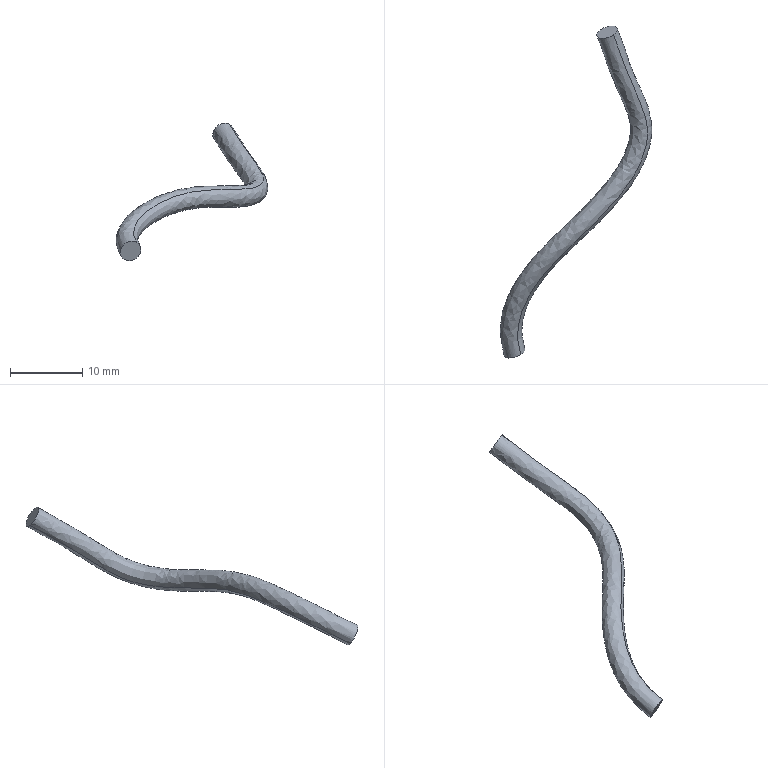Part | SolidWorks | features BaseBody 1 | 1 solid | 4 faces | box 20.926 x 45.783 x 18.973 mm | volume 386.348 mm3 | spline 2 | plane 2
STEP:
#1=CARTESIAN_POINT('',(1917.914,-205.49,926.821));
#2=VERTEX_POINT('',#1);
#3=CARTESIAN_POINT('',(1919.648,-206.093,929.194));
#4=VERTEX_POINT('',#3);
#5=CARTESIAN_POINT('',(1918.781,-205.792,928.008));
#6=DIRECTION('',(-0.2786,0.8622,0.423));
#7=DIRECTION('',(-0.8971,-0.3909,0.206));
#8=AXIS2_PLACEMENT_3D('',#5,#6,#7);
#9=CIRCLE('',#8,1.5);
#10=EDGE_CURVE('',#2,#4,#9,.T.);
#11=ORIENTED_EDGE('',*,*,#10,.T.);
#12=CARTESIAN_POINT('',(1932.433,-161.972,945.472));
#13=VERTEX_POINT('',#12);
#14=CARTESIAN_POINT('',(1919.648,-206.093,929.194));
#15=CARTESIAN_POINT('',(1919.397,-205.314,929.576));
#16=CARTESIAN_POINT('',(1919.227,-204.52,929.968));
#17=CARTESIAN_POINT('',(1919.15,-203.728,930.363));
#18=CARTESIAN_POINT('',(1919.186,-202.087,931.188));
#19=CARTESIAN_POINT('',(1919.601,-200.464,932.011));
#20=CARTESIAN_POINT('',(1919.911,-199.629,932.434));
#21=CARTESIAN_POINT('',(1920.811,-197.733,933.386));
#22=CARTESIAN_POINT('',(1922.058,-195.931,934.252));
#23=CARTESIAN_POINT('',(1922.857,-194.931,934.712));
#24=CARTESIAN_POINT('',(1924.474,-193.116,935.476));
#25=CARTESIAN_POINT('',(1926.3,-191.332,936.005));
#26=CARTESIAN_POINT('',(1927.167,-190.517,936.18));
#27=CARTESIAN_POINT('',(1929.,-188.796,936.417));
#28=CARTESIAN_POINT('',(1930.791,-187.019,936.47));
#29=CARTESIAN_POINT('',(1931.687,-186.078,936.473));
#30=CARTESIAN_POINT('',(1933.237,-184.33,936.474));
#31=CARTESIAN_POINT('',(1934.618,-182.446,936.536));
#32=CARTESIAN_POINT('',(1935.18,-181.584,936.588));
#33=CARTESIAN_POINT('',(1936.101,-179.958,936.744));
#34=CARTESIAN_POINT('',(1936.743,-178.222,937.066));
#35=CARTESIAN_POINT('',(1936.952,-177.433,937.253));
#36=CARTESIAN_POINT('',(1937.175,-176.026,937.663));
#37=CARTESIAN_POINT('',(1937.115,-174.656,938.205));
#38=CARTESIAN_POINT('',(1937.031,-174.042,938.478));
#39=CARTESIAN_POINT('',(1936.759,-172.889,939.053));
#40=CARTESIAN_POINT('',(1936.351,-171.817,939.673));
#41=CARTESIAN_POINT('',(1936.136,-171.318,939.976));
#42=CARTESIAN_POINT('',(1935.572,-170.072,940.747));
#43=CARTESIAN_POINT('',(1935.003,-168.842,941.516));
#44=CARTESIAN_POINT('',(1934.686,-168.106,941.963));
#45=CARTESIAN_POINT('',(1934.027,-166.419,942.951));
#46=CARTESIAN_POINT('',(1933.433,-164.685,943.918));
#47=CARTESIAN_POINT('',(1933.15,-163.847,944.384));
#48=CARTESIAN_POINT('',(1932.801,-162.904,944.925));
#49=CARTESIAN_POINT('',(1932.433,-161.972,945.472));
#50=B_SPLINE_CURVE_WITH_KNOTS('',5,(#14,#15,#16,#17,#18,#19,#20,#21,#22,#23,#24,#25,#26,#27,#28,#29,#30,#31,#32,#33,#34,#35,#36,#37,#38,#39,#40,#41,#42,#43,#44,#45,#46,#47,#48,#49),.UNSPECIFIED.,.F.,.F.,(6,3,3,3,3,3,3,3,3,3,3,6),(0.,0.08786,0.1809,0.3039,0.4114,0.5244,0.617,0.6949,0.759,0.8151,0.8984,1.),.UNSPECIFIED.);
#51=EDGE_CURVE('',#4,#13,#50,.T.);
#52=ORIENTED_EDGE('',*,*,#51,.T.);
#53=CARTESIAN_POINT('',(1930.669,-161.3,943.14));
#54=VERTEX_POINT('',#53);
#55=CARTESIAN_POINT('',(1931.551,-161.636,944.306));
#56=DIRECTION('',(-0.3234,0.8156,0.4797));
#57=DIRECTION('',(-0.8654,-0.4601,0.1988));
#58=AXIS2_PLACEMENT_3D('',#55,#56,#57);
#59=CIRCLE('',#58,1.5);
#60=EDGE_CURVE('',#54,#13,#59,.T.);
#61=ORIENTED_EDGE('',*,*,#60,.F.);
#62=CARTESIAN_POINT('',(1930.669,-161.3,943.14));
#63=CARTESIAN_POINT('',(1931.037,-162.223,942.595));
#64=CARTESIAN_POINT('',(1931.385,-163.158,942.058));
#65=CARTESIAN_POINT('',(1931.668,-163.991,941.594));
#66=CARTESIAN_POINT('',(1932.262,-165.729,940.624));
#67=CARTESIAN_POINT('',(1932.923,-167.438,939.629));
#68=CARTESIAN_POINT('',(1933.241,-168.186,939.178));
#69=CARTESIAN_POINT('',(1933.811,-169.428,938.405));
#70=CARTESIAN_POINT('',(1934.374,-170.663,937.638));
#71=CARTESIAN_POINT('',(1934.588,-171.151,937.339));
#72=CARTESIAN_POINT('',(1934.994,-172.187,936.731));
#73=CARTESIAN_POINT('',(1935.26,-173.283,936.179));
#74=CARTESIAN_POINT('',(1935.338,-173.863,935.921));
#75=CARTESIAN_POINT('',(1935.382,-175.153,935.42));
#76=CARTESIAN_POINT('',(1935.143,-176.466,935.063));
#77=CARTESIAN_POINT('',(1934.928,-177.199,934.906));
#78=CARTESIAN_POINT('',(1934.286,-178.811,934.646));
#79=CARTESIAN_POINT('',(1933.389,-180.326,934.535));
#80=CARTESIAN_POINT('',(1932.845,-181.133,934.502));
#81=CARTESIAN_POINT('',(1931.516,-182.901,934.472));
#82=CARTESIAN_POINT('',(1930.039,-184.548,934.486));
#83=CARTESIAN_POINT('',(1929.19,-185.433,934.487));
#84=CARTESIAN_POINT('',(1927.513,-187.096,934.438));
#85=CARTESIAN_POINT('',(1925.802,-188.705,934.215));
#86=CARTESIAN_POINT('',(1924.987,-189.47,934.052));
#87=CARTESIAN_POINT('',(1923.219,-191.181,933.558));
#88=CARTESIAN_POINT('',(1921.56,-193.001,932.817));
#89=CARTESIAN_POINT('',(1920.716,-194.028,932.36));
#90=CARTESIAN_POINT('',(1919.361,-195.913,931.486));
#91=CARTESIAN_POINT('',(1918.322,-197.986,930.486));
#92=CARTESIAN_POINT('',(1917.949,-198.919,930.034));
#93=CARTESIAN_POINT('',(1917.424,-200.781,929.127));
#94=CARTESIAN_POINT('',(1917.345,-202.722,928.178));
#95=CARTESIAN_POINT('',(1917.427,-203.663,927.718));
#96=CARTESIAN_POINT('',(1917.624,-204.592,927.262));
#97=CARTESIAN_POINT('',(1917.914,-205.49,926.821));
#98=B_SPLINE_CURVE_WITH_KNOTS('',5,(#62,#63,#64,#65,#66,#67,#68,#69,#70,#71,#72,#73,#74,#75,#76,#77,#78,#79,#80,#81,#82,#83,#84,#85,#86,#87,#88,#89,#90,#91,#92,#93,#94,#95,#96,#97),.UNSPECIFIED.,.F.,.F.,(6,3,3,3,3,3,3,3,3,3,3,6),(0.,0.1016,0.1849,0.241,0.3051,0.383,0.4756,0.5886,0.6961,0.8191,0.9121,1.),.UNSPECIFIED.);
#99=EDGE_CURVE('',#54,#2,#98,.T.);
#100=ORIENTED_EDGE('',*,*,#99,.T.);
#101=EDGE_LOOP('',(#11,#52,#61,#100));
#102=FACE_OUTER_BOUND('',#101,.T.);
#103=CARTESIAN_POINT('',(1930.669,-161.3,943.14));
#104=CARTESIAN_POINT('',(1926.22,-164.5,945.581));
#105=CARTESIAN_POINT('',(1931.971,-164.245,949.024));
#106=CARTESIAN_POINT('',(1936.421,-161.045,946.583));
#107=CARTESIAN_POINT('',(1935.119,-158.099,940.699));
#108=CARTESIAN_POINT('',(1930.669,-161.3,943.14));
#109=CARTESIAN_POINT('',(1931.037,-162.223,942.595));
#110=CARTESIAN_POINT('',(1926.553,-165.343,945.079));
#111=CARTESIAN_POINT('',(1932.322,-165.144,948.496));
#112=CARTESIAN_POINT('',(1936.807,-162.024,946.012));
#113=CARTESIAN_POINT('',(1935.521,-159.104,940.112));
#114=CARTESIAN_POINT('',(1931.037,-162.223,942.595));
#115=CARTESIAN_POINT('',(1931.385,-163.158,942.058));
#116=CARTESIAN_POINT('',(1926.864,-166.186,944.59));
#117=CARTESIAN_POINT('',(1932.653,-166.05,947.976));
#118=CARTESIAN_POINT('',(1937.175,-163.022,945.445));
#119=CARTESIAN_POINT('',(1935.906,-160.13,939.526));
#120=CARTESIAN_POINT('',(1931.385,-163.158,942.058));
#121=CARTESIAN_POINT('',(1931.668,-163.991,941.594));
#122=CARTESIAN_POINT('',(1927.127,-166.959,944.156));
#123=CARTESIAN_POINT('',(1932.928,-166.864,947.523));
#124=CARTESIAN_POINT('',(1937.469,-163.895,944.962));
#125=CARTESIAN_POINT('',(1936.209,-161.023,939.032));
#126=CARTESIAN_POINT('',(1931.668,-163.991,941.594));
#127=CARTESIAN_POINT('',(1932.262,-165.729,940.624));
#128=CARTESIAN_POINT('',(1927.74,-168.756,943.157));
#129=CARTESIAN_POINT('',(1933.53,-168.621,946.543));
#130=CARTESIAN_POINT('',(1938.052,-165.595,944.011));
#131=CARTESIAN_POINT('',(1936.785,-162.703,938.092));
#132=CARTESIAN_POINT('',(1932.262,-165.729,940.624));
#133=CARTESIAN_POINT('',(1932.923,-167.438,939.629));
#134=CARTESIAN_POINT('',(1928.496,-170.696,942.04));
#135=CARTESIAN_POINT('',(1934.235,-170.402,945.503));
#136=CARTESIAN_POINT('',(1938.662,-167.144,943.091));
#137=CARTESIAN_POINT('',(1937.351,-164.181,937.218));
#138=CARTESIAN_POINT('',(1932.923,-167.438,939.629));
#139=CARTESIAN_POINT('',(1933.241,-168.186,939.178));
#140=CARTESIAN_POINT('',(1928.867,-171.554,941.529));
#141=CARTESIAN_POINT('',(1934.577,-171.182,945.029));
#142=CARTESIAN_POINT('',(1938.952,-167.814,942.678));
#143=CARTESIAN_POINT('',(1937.615,-164.818,936.827));
#144=CARTESIAN_POINT('',(1933.241,-168.186,939.178));
#145=CARTESIAN_POINT('',(1933.811,-169.428,938.405));
#146=CARTESIAN_POINT('',(1929.495,-172.914,940.691));
#147=CARTESIAN_POINT('',(1935.175,-172.459,944.232));
#148=CARTESIAN_POINT('',(1939.491,-168.973,941.945));
#149=CARTESIAN_POINT('',(1938.127,-165.942,936.118));
#150=CARTESIAN_POINT('',(1933.811,-169.428,938.405));
#151=CARTESIAN_POINT('',(1934.374,-170.663,937.638));
#152=CARTESIAN_POINT('',(1930.003,-174.037,939.986));
#153=CARTESIAN_POINT('',(1935.712,-173.66,943.488));
#154=CARTESIAN_POINT('',(1940.083,-170.286,941.14));
#155=CARTESIAN_POINT('',(1938.745,-167.289,935.29));
#156=CARTESIAN_POINT('',(1934.374,-170.663,937.638));
#157=CARTESIAN_POINT('',(1934.588,-171.151,937.339));
#158=CARTESIAN_POINT('',(1930.168,-174.43,939.739));
#159=CARTESIAN_POINT('',(1935.903,-174.121,943.208));
#160=CARTESIAN_POINT('',(1940.323,-170.843,940.808));
#161=CARTESIAN_POINT('',(1939.008,-167.872,934.938));
#162=CARTESIAN_POINT('',(1934.588,-171.151,937.339));
#163=CARTESIAN_POINT('',(1934.994,-172.187,936.731));
#164=CARTESIAN_POINT('',(1930.408,-175.092,939.331));
#165=CARTESIAN_POINT('',(1936.232,-175.043,942.675));
#166=CARTESIAN_POINT('',(1940.817,-172.138,940.075));
#167=CARTESIAN_POINT('',(1939.579,-169.282,934.131));
#168=CARTESIAN_POINT('',(1934.994,-172.187,936.731));
#169=CARTESIAN_POINT('',(1935.26,-173.283,936.179));
#170=CARTESIAN_POINT('',(1930.491,-175.512,939.107));
#171=CARTESIAN_POINT('',(1936.419,-175.917,942.241));
#172=CARTESIAN_POINT('',(1941.187,-173.688,939.312));
#173=CARTESIAN_POINT('',(1940.028,-171.054,933.25));
#174=CARTESIAN_POINT('',(1935.26,-173.283,936.179));
#175=CARTESIAN_POINT('',(1935.338,-173.863,935.921));
#176=CARTESIAN_POINT('',(1930.505,-175.669,939.041));
#177=CARTESIAN_POINT('',(1936.475,-176.352,942.049));
#178=CARTESIAN_POINT('',(1941.308,-174.546,938.929));
#179=CARTESIAN_POINT('',(1940.17,-172.057,932.801));
#180=CARTESIAN_POINT('',(1935.338,-173.863,935.921));
#181=CARTESIAN_POINT('',(1935.382,-175.153,935.42));
#182=CARTESIAN_POINT('',(1930.528,-175.972,938.951));
#183=CARTESIAN_POINT('',(1936.54,-177.308,941.672));
#184=CARTESIAN_POINT('',(1941.394,-176.489,938.14));
#185=CARTESIAN_POINT('',(1940.236,-174.333,931.888));
#186=CARTESIAN_POINT('',(1935.382,-175.153,935.42));
#187=CARTESIAN_POINT('',(1935.143,-176.466,935.063));
#188=CARTESIAN_POINT('',(1930.508,-176.317,938.934));
#189=CARTESIAN_POINT('',(1936.443,-178.325,941.379));
#190=CARTESIAN_POINT('',(1941.078,-178.475,937.508));
#191=CARTESIAN_POINT('',(1939.778,-176.616,931.191));
#192=CARTESIAN_POINT('',(1935.143,-176.466,935.063));
#193=CARTESIAN_POINT('',(1934.928,-177.199,934.906));
#194=CARTESIAN_POINT('',(1930.478,-176.575,938.923));
#195=CARTESIAN_POINT('',(1936.333,-178.933,941.234));
#196=CARTESIAN_POINT('',(1940.784,-179.557,937.217));
#197=CARTESIAN_POINT('',(1939.379,-177.823,930.889));
#198=CARTESIAN_POINT('',(1934.928,-177.199,934.906));
#199=CARTESIAN_POINT('',(1934.286,-178.811,934.646));
#200=CARTESIAN_POINT('',(1930.27,-177.324,938.903));
#201=CARTESIAN_POINT('',(1935.908,-180.362,940.97));
#202=CARTESIAN_POINT('',(1939.923,-181.849,936.713));
#203=CARTESIAN_POINT('',(1938.302,-180.298,930.388));
#204=CARTESIAN_POINT('',(1934.286,-178.811,934.646));
#205=CARTESIAN_POINT('',(1933.389,-180.326,934.535));
#206=CARTESIAN_POINT('',(1929.775,-178.324,938.902));
#207=CARTESIAN_POINT('',(1935.164,-181.842,940.824));
#208=CARTESIAN_POINT('',(1938.779,-183.844,936.458));
#209=CARTESIAN_POINT('',(1937.004,-182.328,930.168));
#210=CARTESIAN_POINT('',(1933.389,-180.326,934.535));
#211=CARTESIAN_POINT('',(1932.845,-181.133,934.502));
#212=CARTESIAN_POINT('',(1929.415,-178.921,938.909));
#213=CARTESIAN_POINT('',(1934.675,-182.654,940.774));
#214=CARTESIAN_POINT('',(1938.105,-184.866,936.367));
#215=CARTESIAN_POINT('',(1936.275,-183.345,930.095));
#216=CARTESIAN_POINT('',(1932.845,-181.133,934.502));
#217=CARTESIAN_POINT('',(1931.516,-182.901,934.472));
#218=CARTESIAN_POINT('',(1928.43,-180.334,938.943));
#219=CARTESIAN_POINT('',(1933.415,-184.475,940.711));
#220=CARTESIAN_POINT('',(1936.501,-187.042,936.24));
#221=CARTESIAN_POINT('',(1934.602,-185.467,930.002));
#222=CARTESIAN_POINT('',(1931.516,-182.901,934.472));
#223=CARTESIAN_POINT('',(1930.039,-184.548,934.486));
#224=CARTESIAN_POINT('',(1927.129,-181.839,938.98));
#225=CARTESIAN_POINT('',(1931.88,-186.254,940.707));
#226=CARTESIAN_POINT('',(1934.79,-188.963,936.213));
#227=CARTESIAN_POINT('',(1932.949,-187.257,929.991));
#228=CARTESIAN_POINT('',(1930.039,-184.548,934.486));
#229=CARTESIAN_POINT('',(1929.19,-185.433,934.487));
#230=CARTESIAN_POINT('',(1926.328,-182.69,938.99));
#231=CARTESIAN_POINT('',(1930.96,-187.233,940.705));
#232=CARTESIAN_POINT('',(1933.822,-189.977,936.202));
#233=CARTESIAN_POINT('',(1932.052,-188.177,929.984));
#234=CARTESIAN_POINT('',(1929.19,-185.433,934.487));
#235=CARTESIAN_POINT('',(1927.513,-187.096,934.438));
#236=CARTESIAN_POINT('',(1924.631,-184.378,938.947));
#237=CARTESIAN_POINT('',(1929.045,-189.137,940.65));
#238=CARTESIAN_POINT('',(1931.927,-191.854,936.141));
#239=CARTESIAN_POINT('',(1930.395,-189.813,929.928));
#240=CARTESIAN_POINT('',(1927.513,-187.096,934.438));
#241=CARTESIAN_POINT('',(1925.802,-188.705,934.215));
#242=CARTESIAN_POINT('',(1922.685,-186.206,938.695));
#243=CARTESIAN_POINT('',(1926.973,-191.08,940.386));
#244=CARTESIAN_POINT('',(1930.091,-193.579,935.906));
#245=CARTESIAN_POINT('',(1928.92,-191.205,929.734));
#246=CARTESIAN_POINT('',(1925.802,-188.705,934.215));
#247=CARTESIAN_POINT('',(1924.987,-189.47,934.052));
#248=CARTESIAN_POINT('',(1921.706,-187.124,938.505));
#249=CARTESIAN_POINT('',(1925.972,-192.02,940.184));
#250=CARTESIAN_POINT('',(1929.253,-194.366,935.731));
#251=CARTESIAN_POINT('',(1928.268,-191.816,929.599));
#252=CARTESIAN_POINT('',(1924.987,-189.47,934.052));
#253=CARTESIAN_POINT('',(1923.219,-191.181,933.558));
#254=CARTESIAN_POINT('',(1919.572,-189.225,937.925));
#255=CARTESIAN_POINT('',(1923.906,-194.074,939.578));
#256=CARTESIAN_POINT('',(1927.553,-196.03,935.212));
#257=CARTESIAN_POINT('',(1926.866,-193.136,929.191));
#258=CARTESIAN_POINT('',(1923.219,-191.181,933.558));
#259=CARTESIAN_POINT('',(1921.56,-193.001,932.817));
#260=CARTESIAN_POINT('',(1917.581,-191.498,937.065));
#261=CARTESIAN_POINT('',(1922.165,-196.109,938.731));
#262=CARTESIAN_POINT('',(1926.145,-197.612,934.483));
#263=CARTESIAN_POINT('',(1925.539,-194.503,928.568));
#264=CARTESIAN_POINT('',(1921.56,-193.001,932.817));
#265=CARTESIAN_POINT('',(1920.716,-194.028,932.36));
#266=CARTESIAN_POINT('',(1916.579,-192.778,936.541));
#267=CARTESIAN_POINT('',(1921.333,-197.21,938.234));
#268=CARTESIAN_POINT('',(1925.469,-198.46,934.054));
#269=CARTESIAN_POINT('',(1924.852,-195.278,928.18));
#270=CARTESIAN_POINT('',(1920.716,-194.028,932.36));
#271=CARTESIAN_POINT('',(1919.361,-195.913,931.486));
#272=CARTESIAN_POINT('',(1914.956,-195.162,935.526));
#273=CARTESIAN_POINT('',(1920.058,-199.178,937.305));
#274=CARTESIAN_POINT('',(1924.463,-199.929,933.265));
#275=CARTESIAN_POINT('',(1923.766,-196.663,927.446));
#276=CARTESIAN_POINT('',(1919.361,-195.913,931.486));
#277=CARTESIAN_POINT('',(1918.322,-197.986,930.486));
#278=CARTESIAN_POINT('',(1913.687,-197.901,934.316));
#279=CARTESIAN_POINT('',(1919.182,-201.229,936.296));
#280=CARTESIAN_POINT('',(1923.817,-201.315,932.466));
#281=CARTESIAN_POINT('',(1922.958,-198.071,926.657));
#282=CARTESIAN_POINT('',(1918.322,-197.986,930.486));
#283=CARTESIAN_POINT('',(1917.949,-198.919,930.034));
#284=CARTESIAN_POINT('',(1913.224,-199.16,933.754));
#285=CARTESIAN_POINT('',(1918.891,-202.13,935.848));
#286=CARTESIAN_POINT('',(1923.616,-201.889,932.128));
#287=CARTESIAN_POINT('',(1922.674,-198.677,926.313));
#288=CARTESIAN_POINT('',(1917.949,-198.919,930.034));
#289=CARTESIAN_POINT('',(1917.424,-200.781,929.127));
#290=CARTESIAN_POINT('',(1912.576,-201.742,932.59));
#291=CARTESIAN_POINT('',(1918.524,-203.872,934.981));
#292=CARTESIAN_POINT('',(1923.372,-202.912,931.518));
#293=CARTESIAN_POINT('',(1922.272,-199.82,925.664));
#294=CARTESIAN_POINT('',(1917.424,-200.781,929.127));
#295=CARTESIAN_POINT('',(1917.345,-202.722,928.178));
#296=CARTESIAN_POINT('',(1912.513,-204.479,931.315));
#297=CARTESIAN_POINT('',(1918.539,-205.612,934.115));
#298=CARTESIAN_POINT('',(1923.37,-203.855,930.979));
#299=CARTESIAN_POINT('',(1922.177,-200.966,925.042));
#300=CARTESIAN_POINT('',(1917.345,-202.722,928.178));
#301=CARTESIAN_POINT('',(1917.427,-203.663,927.718));
#302=CARTESIAN_POINT('',(1912.646,-205.798,930.687));
#303=CARTESIAN_POINT('',(1918.635,-206.445,933.703));
#304=CARTESIAN_POINT('',(1923.417,-204.309,930.734));
#305=CARTESIAN_POINT('',(1922.209,-201.527,924.749));
#306=CARTESIAN_POINT('',(1917.427,-203.663,927.718));
#307=CARTESIAN_POINT('',(1917.624,-204.592,927.262));
#308=CARTESIAN_POINT('',(1912.923,-207.073,930.069));
#309=CARTESIAN_POINT('',(1918.819,-207.277,933.293));
#310=CARTESIAN_POINT('',(1923.52,-204.795,930.487));
#311=CARTESIAN_POINT('',(1922.324,-202.11,924.456));
#312=CARTESIAN_POINT('',(1917.624,-204.592,927.262));
#313=CARTESIAN_POINT('',(1917.914,-205.49,926.821));
#314=CARTESIAN_POINT('',(1913.312,-208.279,929.475));
#315=CARTESIAN_POINT('',(1919.081,-208.091,932.893));
#316=CARTESIAN_POINT('',(1923.683,-205.303,930.24));
#317=CARTESIAN_POINT('',(1922.516,-202.701,924.168));
#318=CARTESIAN_POINT('',(1917.914,-205.49,926.821));
#319=(BOUNDED_SURFACE()B_SPLINE_SURFACE(5,5,((#103,#104,#105,#106,#107,#108),(#109,#110,#111,#112,#113,#114),(#115,#116,#117,#118,#119,#120),(#121,#122,#123,#124,#125,#126),(#127,#128,#129,#130,#131,#132),(#133,#134,#135,#136,#137,#138),(#139,#140,#141,#142,#143,#144),(#145,#146,#147,#148,#149,#150),(#151,#152,#153,#154,#155,#156),(#157,#158,#159,#160,#161,#162),(#163,#164,#165,#166,#167,#168),(#169,#170,#171,#172,#173,#174),(#175,#176,#177,#178,#179,#180),(#181,#182,#183,#184,#185,#186),(#187,#188,#189,#190,#191,#192),(#193,#194,#195,#196,#197,#198),(#199,#200,#201,#202,#203,#204),(#205,#206,#207,#208,#209,#210),(#211,#212,#213,#214,#215,#216),(#217,#218,#219,#220,#221,#222),(#223,#224,#225,#226,#227,#228),(#229,#230,#231,#232,#233,#234),(#235,#236,#237,#238,#239,#240),(#241,#242,#243,#244,#245,#246),(#247,#248,#249,#250,#251,#252),(#253,#254,#255,#256,#257,#258),(#259,#260,#261,#262,#263,#264),(#265,#266,#267,#268,#269,#270),(#271,#272,#273,#274,#275,#276),(#277,#278,#279,#280,#281,#282),(#283,#284,#285,#286,#287,#288),(#289,#290,#291,#292,#293,#294),(#295,#296,#297,#298,#299,#300),(#301,#302,#303,#304,#305,#306),(#307,#308,#309,#310,#311,#312),(#313,#314,#315,#316,#317,#318)),.UNSPECIFIED.,.F.,.T.,.F.)B_SPLINE_SURFACE_WITH_KNOTS((6,3,3,3,3,3,3,3,3,3,3,6),(6,6),(0.,0.1016,0.1849,0.241,0.3051,0.383,0.4756,0.5886,0.6961,0.8191,0.9121,1.),(0.,1.),.UNSPECIFIED.)GEOMETRIC_REPRESENTATION_ITEM()RATIONAL_B_SPLINE_SURFACE(((1.,0.2,0.2,0.2,0.2,1.),(1.,0.2,0.2,0.2,0.2,1.),(1.,0.2,0.2,0.2,0.2,1.),(1.,0.2,0.2,0.2,0.2,1.),(1.,0.2,0.2,0.2,0.2,1.),(1.,0.2,0.2,0.2,0.2,1.),(1.,0.2,0.2,0.2,0.2,1.),(1.,0.2,0.2,0.2,0.2,1.),(1.,0.2,0.2,0.2,0.2,1.),(1.,0.2,0.2,0.2,0.2,1.),(1.,0.2,0.2,0.2,0.2,1.),(1.,0.2,0.2,0.2,0.2,1.),(1.,0.2,0.2,0.2,0.2,1.),(1.,0.2,0.2,0.2,0.2,1.),(1.,0.2,0.2,0.2,0.2,1.),(1.,0.2,0.2,0.2,0.2,1.),(1.,0.2,0.2,0.2,0.2,1.),(1.,0.2,0.2,0.2,0.2,1.),(1.,0.2,0.2,0.2,0.2,1.),(1.,0.2,0.2,0.2,0.2,1.),(1.,0.2,0.2,0.2,0.2,1.),(1.,0.2,0.2,0.2,0.2,1.),(1.,0.2,0.2,0.2,0.2,1.),(1.,0.2,0.2,0.2,0.2,1.),(1.,0.2,0.2,0.2,0.2,1.),(1.,0.2,0.2,0.2,0.2,1.),(1.,0.2,0.2,0.2,0.2,1.),(1.,0.2,0.2,0.2,0.2,1.),(1.,0.2,0.2,0.2,0.2,1.),(1.,0.2,0.2,0.2,0.2,1.),(1.,0.2,0.2,0.2,0.2,1.),(1.,0.2,0.2,0.2,0.2,1.),(1.,0.2,0.2,0.2,0.2,1.),(1.,0.2,0.2,0.2,0.2,1.),(1.,0.2,0.2,0.2,0.2,1.),(1.,0.2,0.2,0.2,0.2,1.)))REPRESENTATION_ITEM('')SURFACE());
#320=ADVANCED_FACE('',(#102),#319,.T.);
#321=CARTESIAN_POINT('',(1918.781,-205.792,928.008));
#322=DIRECTION('',(-0.2786,0.8622,0.423));
#323=DIRECTION('',(-0.8971,-0.3909,0.206));
#324=AXIS2_PLACEMENT_3D('',#321,#322,#323);
#325=CIRCLE('',#324,1.5);
#326=EDGE_CURVE('',#4,#2,#325,.T.);
#327=ORIENTED_EDGE('',*,*,#326,.T.);
#328=ORIENTED_EDGE('',*,*,#99,.F.);
#329=CARTESIAN_POINT('',(1931.551,-161.636,944.306));
#330=DIRECTION('',(-0.3234,0.8156,0.4797));
#331=DIRECTION('',(-0.8654,-0.4601,0.1988));
#332=AXIS2_PLACEMENT_3D('',#329,#330,#331);
#333=CIRCLE('',#332,1.5);
#334=EDGE_CURVE('',#13,#54,#333,.T.);
#335=ORIENTED_EDGE('',*,*,#334,.F.);
#336=ORIENTED_EDGE('',*,*,#51,.F.);
#337=EDGE_LOOP('',(#327,#328,#335,#336));
#338=FACE_OUTER_BOUND('',#337,.T.);
#339=CARTESIAN_POINT('',(1930.669,-161.3,943.14));
#340=CARTESIAN_POINT('',(1926.22,-164.5,945.581));
#341=CARTESIAN_POINT('',(1931.971,-164.245,949.024));
#342=CARTESIAN_POINT('',(1936.421,-161.045,946.583));
#343=CARTESIAN_POINT('',(1935.119,-158.099,940.699));
#344=CARTESIAN_POINT('',(1930.669,-161.3,943.14));
#345=CARTESIAN_POINT('',(1931.037,-162.223,942.595));
#346=CARTESIAN_POINT('',(1926.553,-165.343,945.079));
#347=CARTESIAN_POINT('',(1932.322,-165.144,948.496));
#348=CARTESIAN_POINT('',(1936.807,-162.024,946.012));
#349=CARTESIAN_POINT('',(1935.521,-159.104,940.112));
#350=CARTESIAN_POINT('',(1931.037,-162.223,942.595));
#351=CARTESIAN_POINT('',(1931.385,-163.158,942.058));
#352=CARTESIAN_POINT('',(1926.864,-166.186,944.59));
#353=CARTESIAN_POINT('',(1932.653,-166.05,947.976));
#354=CARTESIAN_POINT('',(1937.175,-163.022,945.445));
#355=CARTESIAN_POINT('',(1935.906,-160.13,939.526));
#356=CARTESIAN_POINT('',(1931.385,-163.158,942.058));
#357=CARTESIAN_POINT('',(1931.668,-163.991,941.594));
#358=CARTESIAN_POINT('',(1927.127,-166.959,944.156));
#359=CARTESIAN_POINT('',(1932.928,-166.864,947.523));
#360=CARTESIAN_POINT('',(1937.469,-163.895,944.962));
#361=CARTESIAN_POINT('',(1936.209,-161.023,939.032));
#362=CARTESIAN_POINT('',(1931.668,-163.991,941.594));
#363=CARTESIAN_POINT('',(1932.262,-165.729,940.624));
#364=CARTESIAN_POINT('',(1927.74,-168.756,943.157));
#365=CARTESIAN_POINT('',(1933.53,-168.621,946.543));
#366=CARTESIAN_POINT('',(1938.052,-165.595,944.011));
#367=CARTESIAN_POINT('',(1936.785,-162.703,938.092));
#368=CARTESIAN_POINT('',(1932.262,-165.729,940.624));
#369=CARTESIAN_POINT('',(1932.923,-167.438,939.629));
#370=CARTESIAN_POINT('',(1928.496,-170.696,942.04));
#371=CARTESIAN_POINT('',(1934.235,-170.402,945.503));
#372=CARTESIAN_POINT('',(1938.662,-167.144,943.091));
#373=CARTESIAN_POINT('',(1937.351,-164.181,937.218));
#374=CARTESIAN_POINT('',(1932.923,-167.438,939.629));
#375=CARTESIAN_POINT('',(1933.241,-168.186,939.178));
#376=CARTESIAN_POINT('',(1928.867,-171.554,941.529));
#377=CARTESIAN_POINT('',(1934.577,-171.182,945.029));
#378=CARTESIAN_POINT('',(1938.952,-167.814,942.678));
#379=CARTESIAN_POINT('',(1937.615,-164.818,936.827));
#380=CARTESIAN_POINT('',(1933.241,-168.186,939.178));
#381=CARTESIAN_POINT('',(1933.811,-169.428,938.405));
#382=CARTESIAN_POINT('',(1929.495,-172.914,940.691));
#383=CARTESIAN_POINT('',(1935.175,-172.459,944.232));
#384=CARTESIAN_POINT('',(1939.491,-168.973,941.945));
#385=CARTESIAN_POINT('',(1938.127,-165.942,936.118));
#386=CARTESIAN_POINT('',(1933.811,-169.428,938.405));
#387=CARTESIAN_POINT('',(1934.374,-170.663,937.638));
#388=CARTESIAN_POINT('',(1930.003,-174.037,939.986));
#389=CARTESIAN_POINT('',(1935.712,-173.66,943.488));
#390=CARTESIAN_POINT('',(1940.083,-170.286,941.14));
#391=CARTESIAN_POINT('',(1938.745,-167.289,935.29));
#392=CARTESIAN_POINT('',(1934.374,-170.663,937.638));
#393=CARTESIAN_POINT('',(1934.588,-171.151,937.339));
#394=CARTESIAN_POINT('',(1930.168,-174.43,939.739));
#395=CARTESIAN_POINT('',(1935.903,-174.121,943.208));
#396=CARTESIAN_POINT('',(1940.323,-170.843,940.808));
#397=CARTESIAN_POINT('',(1939.008,-167.872,934.938));
#398=CARTESIAN_POINT('',(1934.588,-171.151,937.339));
#399=CARTESIAN_POINT('',(1934.994,-172.187,936.731));
#400=CARTESIAN_POINT('',(1930.408,-175.092,939.331));
#401=CARTESIAN_POINT('',(1936.232,-175.043,942.675));
#402=CARTESIAN_POINT('',(1940.817,-172.138,940.075));
#403=CARTESIAN_POINT('',(1939.579,-169.282,934.131));
#404=CARTESIAN_POINT('',(1934.994,-172.187,936.731));
#405=CARTESIAN_POINT('',(1935.26,-173.283,936.179));
#406=CARTESIAN_POINT('',(1930.491,-175.512,939.107));
#407=CARTESIAN_POINT('',(1936.419,-175.917,942.241));
#408=CARTESIAN_POINT('',(1941.187,-173.688,939.312));
#409=CARTESIAN_POINT('',(1940.028,-171.054,933.25));
#410=CARTESIAN_POINT('',(1935.26,-173.283,936.179));
#411=CARTESIAN_POINT('',(1935.338,-173.863,935.921));
#412=CARTESIAN_POINT('',(1930.505,-175.669,939.041));
#413=CARTESIAN_POINT('',(1936.475,-176.352,942.049));
#414=CARTESIAN_POINT('',(1941.308,-174.546,938.929));
#415=CARTESIAN_POINT('',(1940.17,-172.057,932.801));
#416=CARTESIAN_POINT('',(1935.338,-173.863,935.921));
#417=CARTESIAN_POINT('',(1935.382,-175.153,935.42));
#418=CARTESIAN_POINT('',(1930.528,-175.972,938.951));
#419=CARTESIAN_POINT('',(1936.54,-177.308,941.672));
#420=CARTESIAN_POINT('',(1941.394,-176.489,938.14));
#421=CARTESIAN_POINT('',(1940.236,-174.333,931.888));
#422=CARTESIAN_POINT('',(1935.382,-175.153,935.42));
#423=CARTESIAN_POINT('',(1935.143,-176.466,935.063));
#424=CARTESIAN_POINT('',(1930.508,-176.317,938.934));
#425=CARTESIAN_POINT('',(1936.443,-178.325,941.379));
#426=CARTESIAN_POINT('',(1941.078,-178.475,937.508));
#427=CARTESIAN_POINT('',(1939.778,-176.616,931.191));
#428=CARTESIAN_POINT('',(1935.143,-176.466,935.063));
#429=CARTESIAN_POINT('',(1934.928,-177.199,934.906));
#430=CARTESIAN_POINT('',(1930.478,-176.575,938.923));
#431=CARTESIAN_POINT('',(1936.333,-178.933,941.234));
#432=CARTESIAN_POINT('',(1940.784,-179.557,937.217));
#433=CARTESIAN_POINT('',(1939.379,-177.823,930.889));
#434=CARTESIAN_POINT('',(1934.928,-177.199,934.906));
#435=CARTESIAN_POINT('',(1934.286,-178.811,934.646));
#436=CARTESIAN_POINT('',(1930.27,-177.324,938.903));
#437=CARTESIAN_POINT('',(1935.908,-180.362,940.97));
#438=CARTESIAN_POINT('',(1939.923,-181.849,936.713));
#439=CARTESIAN_POINT('',(1938.302,-180.298,930.388));
#440=CARTESIAN_POINT('',(1934.286,-178.811,934.646));
#441=CARTESIAN_POINT('',(1933.389,-180.326,934.535));
#442=CARTESIAN_POINT('',(1929.775,-178.324,938.902));
#443=CARTESIAN_POINT('',(1935.164,-181.842,940.824));
#444=CARTESIAN_POINT('',(1938.779,-183.844,936.458));
#445=CARTESIAN_POINT('',(1937.004,-182.328,930.168));
#446=CARTESIAN_POINT('',(1933.389,-180.326,934.535));
#447=CARTESIAN_POINT('',(1932.845,-181.133,934.502));
#448=CARTESIAN_POINT('',(1929.415,-178.921,938.909));
#449=CARTESIAN_POINT('',(1934.675,-182.654,940.774));
#450=CARTESIAN_POINT('',(1938.105,-184.866,936.367));
#451=CARTESIAN_POINT('',(1936.275,-183.345,930.095));
#452=CARTESIAN_POINT('',(1932.845,-181.133,934.502));
#453=CARTESIAN_POINT('',(1931.516,-182.901,934.472));
#454=CARTESIAN_POINT('',(1928.43,-180.334,938.943));
#455=CARTESIAN_POINT('',(1933.415,-184.475,940.711));
#456=CARTESIAN_POINT('',(1936.501,-187.042,936.24));
#457=CARTESIAN_POINT('',(1934.602,-185.467,930.002));
#458=CARTESIAN_POINT('',(1931.516,-182.901,934.472));
#459=CARTESIAN_POINT('',(1930.039,-184.548,934.486));
#460=CARTESIAN_POINT('',(1927.129,-181.839,938.98));
#461=CARTESIAN_POINT('',(1931.88,-186.254,940.707));
#462=CARTESIAN_POINT('',(1934.79,-188.963,936.213));
#463=CARTESIAN_POINT('',(1932.949,-187.257,929.991));
#464=CARTESIAN_POINT('',(1930.039,-184.548,934.486));
#465=CARTESIAN_POINT('',(1929.19,-185.433,934.487));
#466=CARTESIAN_POINT('',(1926.328,-182.69,938.99));
#467=CARTESIAN_POINT('',(1930.96,-187.233,940.705));
#468=CARTESIAN_POINT('',(1933.822,-189.977,936.202));
#469=CARTESIAN_POINT('',(1932.052,-188.177,929.984));
#470=CARTESIAN_POINT('',(1929.19,-185.433,934.487));
#471=CARTESIAN_POINT('',(1927.513,-187.096,934.438));
#472=CARTESIAN_POINT('',(1924.631,-184.378,938.947));
#473=CARTESIAN_POINT('',(1929.045,-189.137,940.65));
#474=CARTESIAN_POINT('',(1931.927,-191.854,936.141));
#475=CARTESIAN_POINT('',(1930.395,-189.813,929.928));
#476=CARTESIAN_POINT('',(1927.513,-187.096,934.438));
#477=CARTESIAN_POINT('',(1925.802,-188.705,934.215));
#478=CARTESIAN_POINT('',(1922.685,-186.206,938.695));
#479=CARTESIAN_POINT('',(1926.973,-191.08,940.386));
#480=CARTESIAN_POINT('',(1930.091,-193.579,935.906));
#481=CARTESIAN_POINT('',(1928.92,-191.205,929.734));
#482=CARTESIAN_POINT('',(1925.802,-188.705,934.215));
#483=CARTESIAN_POINT('',(1924.987,-189.47,934.052));
#484=CARTESIAN_POINT('',(1921.706,-187.124,938.505));
#485=CARTESIAN_POINT('',(1925.972,-192.02,940.184));
#486=CARTESIAN_POINT('',(1929.253,-194.366,935.731));
#487=CARTESIAN_POINT('',(1928.268,-191.816,929.599));
#488=CARTESIAN_POINT('',(1924.987,-189.47,934.052));
#489=CARTESIAN_POINT('',(1923.219,-191.181,933.558));
#490=CARTESIAN_POINT('',(1919.572,-189.225,937.925));
#491=CARTESIAN_POINT('',(1923.906,-194.074,939.578));
#492=CARTESIAN_POINT('',(1927.553,-196.03,935.212));
#493=CARTESIAN_POINT('',(1926.866,-193.136,929.191));
#494=CARTESIAN_POINT('',(1923.219,-191.181,933.558));
#495=CARTESIAN_POINT('',(1921.56,-193.001,932.817));
#496=CARTESIAN_POINT('',(1917.581,-191.498,937.065));
#497=CARTESIAN_POINT('',(1922.165,-196.109,938.731));
#498=CARTESIAN_POINT('',(1926.145,-197.612,934.483));
#499=CARTESIAN_POINT('',(1925.539,-194.503,928.568));
#500=CARTESIAN_POINT('',(1921.56,-193.001,932.817));
#501=CARTESIAN_POINT('',(1920.716,-194.028,932.36));
#502=CARTESIAN_POINT('',(1916.579,-192.778,936.541));
#503=CARTESIAN_POINT('',(1921.333,-197.21,938.234));
#504=CARTESIAN_POINT('',(1925.469,-198.46,934.054));
#505=CARTESIAN_POINT('',(1924.852,-195.278,928.18));
#506=CARTESIAN_POINT('',(1920.716,-194.028,932.36));
#507=CARTESIAN_POINT('',(1919.361,-195.913,931.486));
#508=CARTESIAN_POINT('',(1914.956,-195.162,935.526));
#509=CARTESIAN_POINT('',(1920.058,-199.178,937.305));
#510=CARTESIAN_POINT('',(1924.463,-199.929,933.265));
#511=CARTESIAN_POINT('',(1923.766,-196.663,927.446));
#512=CARTESIAN_POINT('',(1919.361,-195.913,931.486));
#513=CARTESIAN_POINT('',(1918.322,-197.986,930.486));
#514=CARTESIAN_POINT('',(1913.687,-197.901,934.316));
#515=CARTESIAN_POINT('',(1919.182,-201.229,936.296));
#516=CARTESIAN_POINT('',(1923.817,-201.315,932.466));
#517=CARTESIAN_POINT('',(1922.958,-198.071,926.657));
#518=CARTESIAN_POINT('',(1918.322,-197.986,930.486));
#519=CARTESIAN_POINT('',(1917.949,-198.919,930.034));
#520=CARTESIAN_POINT('',(1913.224,-199.16,933.754));
#521=CARTESIAN_POINT('',(1918.891,-202.13,935.848));
#522=CARTESIAN_POINT('',(1923.616,-201.889,932.128));
#523=CARTESIAN_POINT('',(1922.674,-198.677,926.313));
#524=CARTESIAN_POINT('',(1917.949,-198.919,930.034));
#525=CARTESIAN_POINT('',(1917.424,-200.781,929.127));
#526=CARTESIAN_POINT('',(1912.576,-201.742,932.59));
#527=CARTESIAN_POINT('',(1918.524,-203.872,934.981));
#528=CARTESIAN_POINT('',(1923.372,-202.912,931.518));
#529=CARTESIAN_POINT('',(1922.272,-199.82,925.664));
#530=CARTESIAN_POINT('',(1917.424,-200.781,929.127));
#531=CARTESIAN_POINT('',(1917.345,-202.722,928.178));
#532=CARTESIAN_POINT('',(1912.513,-204.479,931.315));
#533=CARTESIAN_POINT('',(1918.539,-205.612,934.115));
#534=CARTESIAN_POINT('',(1923.37,-203.855,930.979));
#535=CARTESIAN_POINT('',(1922.177,-200.966,925.042));
#536=CARTESIAN_POINT('',(1917.345,-202.722,928.178));
#537=CARTESIAN_POINT('',(1917.427,-203.663,927.718));
#538=CARTESIAN_POINT('',(1912.646,-205.798,930.687));
#539=CARTESIAN_POINT('',(1918.635,-206.445,933.703));
#540=CARTESIAN_POINT('',(1923.417,-204.309,930.734));
#541=CARTESIAN_POINT('',(1922.209,-201.527,924.749));
#542=CARTESIAN_POINT('',(1917.427,-203.663,927.718));
#543=CARTESIAN_POINT('',(1917.624,-204.592,927.262));
#544=CARTESIAN_POINT('',(1912.923,-207.073,930.069));
#545=CARTESIAN_POINT('',(1918.819,-207.277,933.293));
#546=CARTESIAN_POINT('',(1923.52,-204.795,930.487));
#547=CARTESIAN_POINT('',(1922.324,-202.11,924.456));
#548=CARTESIAN_POINT('',(1917.624,-204.592,927.262));
#549=CARTESIAN_POINT('',(1917.914,-205.49,926.821));
#550=CARTESIAN_POINT('',(1913.312,-208.279,929.475));
#551=CARTESIAN_POINT('',(1919.081,-208.091,932.893));
#552=CARTESIAN_POINT('',(1923.683,-205.303,930.24));
#553=CARTESIAN_POINT('',(1922.516,-202.701,924.168));
#554=CARTESIAN_POINT('',(1917.914,-205.49,926.821));
#555=(BOUNDED_SURFACE()B_SPLINE_SURFACE(5,5,((#339,#340,#341,#342,#343,#344),(#345,#346,#347,#348,#349,#350),(#351,#352,#353,#354,#355,#356),(#357,#358,#359,#360,#361,#362),(#363,#364,#365,#366,#367,#368),(#369,#370,#371,#372,#373,#374),(#375,#376,#377,#378,#379,#380),(#381,#382,#383,#384,#385,#386),(#387,#388,#389,#390,#391,#392),(#393,#394,#395,#396,#397,#398),(#399,#400,#401,#402,#403,#404),(#405,#406,#407,#408,#409,#410),(#411,#412,#413,#414,#415,#416),(#417,#418,#419,#420,#421,#422),(#423,#424,#425,#426,#427,#428),(#429,#430,#431,#432,#433,#434),(#435,#436,#437,#438,#439,#440),(#441,#442,#443,#444,#445,#446),(#447,#448,#449,#450,#451,#452),(#453,#454,#455,#456,#457,#458),(#459,#460,#461,#462,#463,#464),(#465,#466,#467,#468,#469,#470),(#471,#472,#473,#474,#475,#476),(#477,#478,#479,#480,#481,#482),(#483,#484,#485,#486,#487,#488),(#489,#490,#491,#492,#493,#494),(#495,#496,#497,#498,#499,#500),(#501,#502,#503,#504,#505,#506),(#507,#508,#509,#510,#511,#512),(#513,#514,#515,#516,#517,#518),(#519,#520,#521,#522,#523,#524),(#525,#526,#527,#528,#529,#530),(#531,#532,#533,#534,#535,#536),(#537,#538,#539,#540,#541,#542),(#543,#544,#545,#546,#547,#548),(#549,#550,#551,#552,#553,#554)),.UNSPECIFIED.,.F.,.T.,.F.)B_SPLINE_SURFACE_WITH_KNOTS((6,3,3,3,3,3,3,3,3,3,3,6),(6,6),(0.,0.1016,0.1849,0.241,0.3051,0.383,0.4756,0.5886,0.6961,0.8191,0.9121,1.),(0.,1.),.UNSPECIFIED.)GEOMETRIC_REPRESENTATION_ITEM()RATIONAL_B_SPLINE_SURFACE(((1.,0.2,0.2,0.2,0.2,1.),(1.,0.2,0.2,0.2,0.2,1.),(1.,0.2,0.2,0.2,0.2,1.),(1.,0.2,0.2,0.2,0.2,1.),(1.,0.2,0.2,0.2,0.2,1.),(1.,0.2,0.2,0.2,0.2,1.),(1.,0.2,0.2,0.2,0.2,1.),(1.,0.2,0.2,0.2,0.2,1.),(1.,0.2,0.2,0.2,0.2,1.),(1.,0.2,0.2,0.2,0.2,1.),(1.,0.2,0.2,0.2,0.2,1.),(1.,0.2,0.2,0.2,0.2,1.),(1.,0.2,0.2,0.2,0.2,1.),(1.,0.2,0.2,0.2,0.2,1.),(1.,0.2,0.2,0.2,0.2,1.),(1.,0.2,0.2,0.2,0.2,1.),(1.,0.2,0.2,0.2,0.2,1.),(1.,0.2,0.2,0.2,0.2,1.),(1.,0.2,0.2,0.2,0.2,1.),(1.,0.2,0.2,0.2,0.2,1.),(1.,0.2,0.2,0.2,0.2,1.),(1.,0.2,0.2,0.2,0.2,1.),(1.,0.2,0.2,0.2,0.2,1.),(1.,0.2,0.2,0.2,0.2,1.),(1.,0.2,0.2,0.2,0.2,1.),(1.,0.2,0.2,0.2,0.2,1.),(1.,0.2,0.2,0.2,0.2,1.),(1.,0.2,0.2,0.2,0.2,1.),(1.,0.2,0.2,0.2,0.2,1.),(1.,0.2,0.2,0.2,0.2,1.),(1.,0.2,0.2,0.2,0.2,1.),(1.,0.2,0.2,0.2,0.2,1.),(1.,0.2,0.2,0.2,0.2,1.),(1.,0.2,0.2,0.2,0.2,1.),(1.,0.2,0.2,0.2,0.2,1.),(1.,0.2,0.2,0.2,0.2,1.)))REPRESENTATION_ITEM('')SURFACE());
#556=ADVANCED_FACE('',(#338),#555,.T.);
#557=ORIENTED_EDGE('',*,*,#60,.T.);
#558=ORIENTED_EDGE('',*,*,#334,.T.);
#559=EDGE_LOOP('',(#557,#558));
#560=FACE_OUTER_BOUND('',#559,.T.);
#561=CARTESIAN_POINT('',(1900.939,-129.204,868.53));
#562=DIRECTION('',(-0.3234,0.8156,0.4797));
#563=DIRECTION('',(-0.5877,0.2242,-0.7774));
#564=AXIS2_PLACEMENT_3D('',#561,#562,#563);
#565=PLANE('',#564);
#566=ADVANCED_FACE('',(#560),#565,.T.);
#567=ORIENTED_EDGE('',*,*,#326,.F.);
#568=ORIENTED_EDGE('',*,*,#10,.F.);
#569=EDGE_LOOP('',(#567,#568));
#570=FACE_OUTER_BOUND('',#569,.T.);
#571=CARTESIAN_POINT('',(1889.634,-177.037,850.197));
#572=DIRECTION('',(-0.2786,0.8622,0.423));
#573=DIRECTION('',(-0.578,0.2012,-0.7908));
#574=AXIS2_PLACEMENT_3D('',#571,#572,#573);
#575=PLANE('',#574);
#576=ADVANCED_FACE('',(#570),#575,.F.);
#577=CLOSED_SHELL('',(#320,#556,#566,#576));
#578=MANIFOLD_SOLID_BREP('',#577);
#579=CARTESIAN_POINT('',(0.,0.,0.));
#580=DIRECTION('',(0.,0.,1.));
#581=DIRECTION('',(1.,0.,0.));
#582=AXIS2_PLACEMENT_3D('',#579,#580,#581);
#583=(LENGTH_UNIT()NAMED_UNIT(*)SI_UNIT(.MILLI.,.METRE.));
#584=UNCERTAINTY_MEASURE_WITH_UNIT(LENGTH_MEASURE(0.00001),#583,'','');
#585=(NAMED_UNIT(*)PLANE_ANGLE_UNIT()SI_UNIT($,.RADIAN.));
#586=(NAMED_UNIT(*)SI_UNIT($,.STERADIAN.)SOLID_ANGLE_UNIT());
#587=(GEOMETRIC_REPRESENTATION_CONTEXT(3)GLOBAL_UNCERTAINTY_ASSIGNED_CONTEXT((#584))GLOBAL_UNIT_ASSIGNED_CONTEXT((#583,#585,#586))REPRESENTATION_CONTEXT('',''));
#588=ADVANCED_BREP_SHAPE_REPRESENTATION('',(#578,#582),#587);